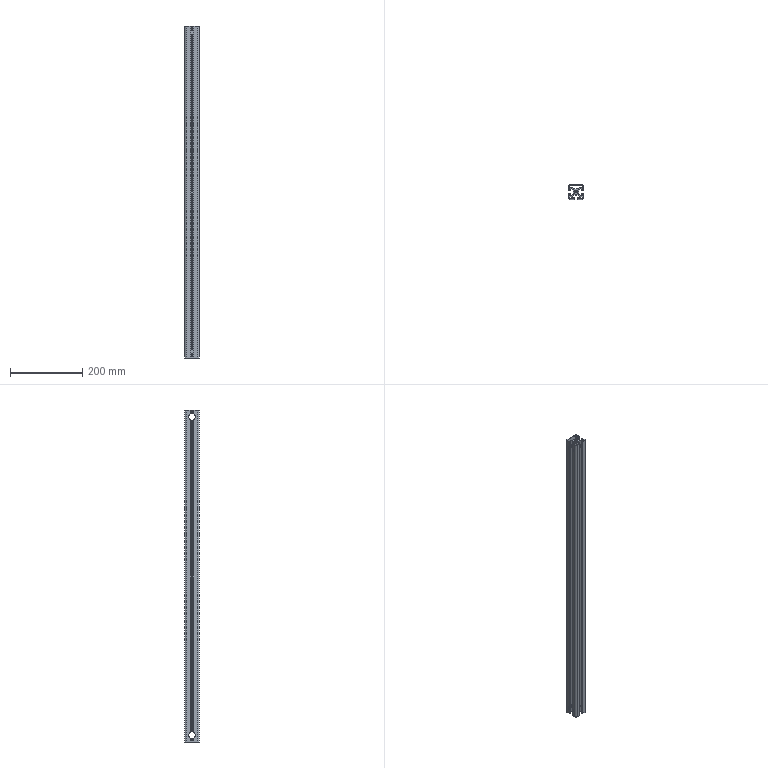Part | SolidWorks | features BaseBody 1, HoleWzd 1, MoveFace 1 | 1 solid | 242 faces | box 40 x 40 x 920 mm | volume 536323 mm3 | plane 187 | cylinder 55 | commonest cylinder face diameters 6.8 x15 2 x14 19 x12 1 x6 5 x4 9 x4